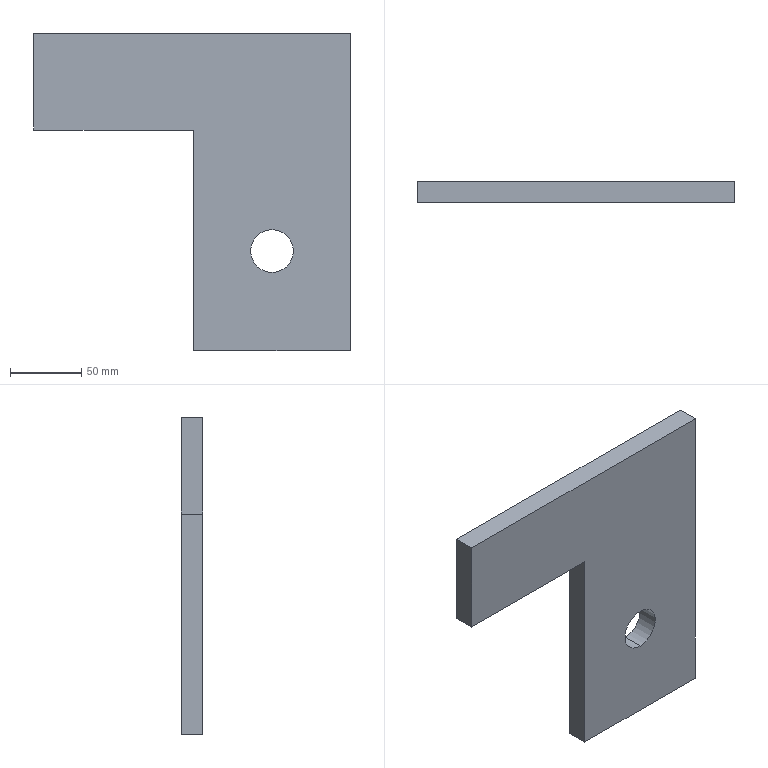Part | SolidWorks | features BaseBody 1 | 1 solid | 10 faces | box 222.333 x 15 x 223.043 mm | volume 471998 mm3 | plane 8 | cylinder 2 | commonest cylinder face diameters 30 x2
STEP:
#1=CARTESIAN_POINT('',(57.247,354.5,-81.));
#2=VERTEX_POINT('',#1);
#3=CARTESIAN_POINT('',(57.247,354.5,-51.));
#4=VERTEX_POINT('',#3);
#5=CARTESIAN_POINT('',(57.247,354.5,-66.));
#6=DIRECTION('',(0.,1.,0.));
#7=DIRECTION('',(0.,0.,1.));
#8=AXIS2_PLACEMENT_3D('',#5,#6,#7);
#9=CIRCLE('',#8,15.);
#10=EDGE_CURVE('',#2,#4,#9,.T.);
#11=ORIENTED_EDGE('',*,*,#10,.F.);
#12=CARTESIAN_POINT('',(57.247,369.5,-81.));
#13=VERTEX_POINT('',#12);
#14=CARTESIAN_POINT('',(57.247,389.5,-81.));
#15=DIRECTION('',(0.,1.,0.));
#16=VECTOR('',#15,1000.);
#17=LINE('',#14,#16);
#18=EDGE_CURVE('',#2,#13,#17,.T.);
#19=ORIENTED_EDGE('',*,*,#18,.T.);
#20=CARTESIAN_POINT('',(57.247,369.5,-51.));
#21=VERTEX_POINT('',#20);
#22=CARTESIAN_POINT('',(57.247,369.5,-66.));
#23=DIRECTION('',(0.,-1.,0.));
#24=DIRECTION('',(0.,0.,1.));
#25=AXIS2_PLACEMENT_3D('',#22,#23,#24);
#26=CIRCLE('',#25,15.);
#27=EDGE_CURVE('',#21,#13,#26,.T.);
#28=ORIENTED_EDGE('',*,*,#27,.F.);
#29=CARTESIAN_POINT('',(57.247,389.5,-51.));
#30=DIRECTION('',(0.,1.,0.));
#31=VECTOR('',#30,1000.);
#32=LINE('',#29,#31);
#33=EDGE_CURVE('',#4,#21,#32,.T.);
#34=ORIENTED_EDGE('',*,*,#33,.F.);
#35=EDGE_LOOP('',(#11,#19,#28,#34));
#36=FACE_OUTER_BOUND('',#35,.T.);
#37=CARTESIAN_POINT('',(57.247,389.5,-66.));
#38=DIRECTION('',(0.,1.,0.));
#39=DIRECTION('',(0.,0.,1.));
#40=AXIS2_PLACEMENT_3D('',#37,#38,#39);
#41=CYLINDRICAL_SURFACE('',#40,15.);
#42=ADVANCED_FACE('',(#36),#41,.F.);
#43=ORIENTED_EDGE('',*,*,#27,.T.);
#44=CARTESIAN_POINT('',(57.247,369.5,-66.));
#45=DIRECTION('',(0.,-1.,0.));
#46=DIRECTION('',(0.,0.,1.));
#47=AXIS2_PLACEMENT_3D('',#44,#45,#46);
#48=CIRCLE('',#47,15.);
#49=EDGE_CURVE('',#13,#21,#48,.T.);
#50=ORIENTED_EDGE('',*,*,#49,.T.);
#51=EDGE_LOOP('',(#43,#50));
#52=FACE_BOUND('',#51,.T.);
#53=CARTESIAN_POINT('',(112.247,369.5,-136.043));
#54=VERTEX_POINT('',#53);
#55=CARTESIAN_POINT('',(2.247,369.5,-136.043));
#56=VERTEX_POINT('',#55);
#57=CARTESIAN_POINT('',(57.247,369.5,-136.043));
#58=DIRECTION('',(-1.,0.,0.));
#59=VECTOR('',#58,1000.);
#60=LINE('',#57,#59);
#61=EDGE_CURVE('',#54,#56,#60,.T.);
#62=ORIENTED_EDGE('',*,*,#61,.T.);
#63=CARTESIAN_POINT('',(2.247,369.5,19.));
#64=VERTEX_POINT('',#63);
#65=CARTESIAN_POINT('',(2.247,369.5,-16.043));
#66=DIRECTION('',(0.,0.,1.));
#67=VECTOR('',#66,1000.);
#68=LINE('',#65,#67);
#69=EDGE_CURVE('',#56,#64,#68,.T.);
#70=ORIENTED_EDGE('',*,*,#69,.T.);
#71=CARTESIAN_POINT('',(-110.086,369.5,19.));
#72=VERTEX_POINT('',#71);
#73=CARTESIAN_POINT('',(57.247,369.5,19.));
#74=DIRECTION('',(-1.,0.,0.));
#75=VECTOR('',#74,1000.);
#76=LINE('',#73,#75);
#77=EDGE_CURVE('',#64,#72,#76,.T.);
#78=ORIENTED_EDGE('',*,*,#77,.T.);
#79=CARTESIAN_POINT('',(-110.086,369.5,87.));
#80=VERTEX_POINT('',#79);
#81=CARTESIAN_POINT('',(-110.086,369.5,-16.043));
#82=DIRECTION('',(0.,0.,1.));
#83=VECTOR('',#82,1000.);
#84=LINE('',#81,#83);
#85=EDGE_CURVE('',#72,#80,#84,.T.);
#86=ORIENTED_EDGE('',*,*,#85,.T.);
#87=CARTESIAN_POINT('',(112.247,369.5,87.));
#88=VERTEX_POINT('',#87);
#89=CARTESIAN_POINT('',(57.247,369.5,87.));
#90=DIRECTION('',(1.,0.,0.));
#91=VECTOR('',#90,1000.);
#92=LINE('',#89,#91);
#93=EDGE_CURVE('',#80,#88,#92,.T.);
#94=ORIENTED_EDGE('',*,*,#93,.T.);
#95=CARTESIAN_POINT('',(112.247,369.5,-16.043));
#96=DIRECTION('',(0.,0.,-1.));
#97=VECTOR('',#96,1000.);
#98=LINE('',#95,#97);
#99=EDGE_CURVE('',#88,#54,#98,.T.);
#100=ORIENTED_EDGE('',*,*,#99,.T.);
#101=EDGE_LOOP('',(#62,#70,#78,#86,#94,#100));
#102=FACE_OUTER_BOUND('',#101,.T.);
#103=CARTESIAN_POINT('',(57.247,369.5,-16.043));
#104=DIRECTION('',(0.,1.,0.));
#105=DIRECTION('',(0.,0.,1.));
#106=AXIS2_PLACEMENT_3D('',#103,#104,#105);
#107=PLANE('',#106);
#108=ADVANCED_FACE('',(#52,#102),#107,.T.);
#109=ORIENTED_EDGE('',*,*,#18,.F.);
#110=CARTESIAN_POINT('',(57.247,354.5,-66.));
#111=DIRECTION('',(0.,1.,0.));
#112=DIRECTION('',(0.,0.,1.));
#113=AXIS2_PLACEMENT_3D('',#110,#111,#112);
#114=CIRCLE('',#113,15.);
#115=EDGE_CURVE('',#4,#2,#114,.T.);
#116=ORIENTED_EDGE('',*,*,#115,.F.);
#117=ORIENTED_EDGE('',*,*,#33,.T.);
#118=ORIENTED_EDGE('',*,*,#49,.F.);
#119=EDGE_LOOP('',(#109,#116,#117,#118));
#120=FACE_OUTER_BOUND('',#119,.T.);
#121=CARTESIAN_POINT('',(57.247,389.5,-66.));
#122=DIRECTION('',(0.,1.,0.));
#123=DIRECTION('',(0.,0.,1.));
#124=AXIS2_PLACEMENT_3D('',#121,#122,#123);
#125=CYLINDRICAL_SURFACE('',#124,15.);
#126=ADVANCED_FACE('',(#120),#125,.F.);
#127=CARTESIAN_POINT('',(2.247,354.5,-136.043));
#128=VERTEX_POINT('',#127);
#129=CARTESIAN_POINT('',(2.247,354.5,19.));
#130=VERTEX_POINT('',#129);
#131=CARTESIAN_POINT('',(2.247,354.5,-16.043));
#132=DIRECTION('',(0.,0.,1.));
#133=VECTOR('',#132,1000.);
#134=LINE('',#131,#133);
#135=EDGE_CURVE('',#128,#130,#134,.T.);
#136=ORIENTED_EDGE('',*,*,#135,.T.);
#137=CARTESIAN_POINT('',(2.247,357.,19.));
#138=DIRECTION('',(0.,1.,0.));
#139=VECTOR('',#138,1000.);
#140=LINE('',#137,#139);
#141=EDGE_CURVE('',#130,#64,#140,.T.);
#142=ORIENTED_EDGE('',*,*,#141,.T.);
#143=ORIENTED_EDGE('',*,*,#69,.F.);
#144=CARTESIAN_POINT('',(2.247,357.,-136.043));
#145=DIRECTION('',(0.,-1.,0.));
#146=VECTOR('',#145,1000.);
#147=LINE('',#144,#146);
#148=EDGE_CURVE('',#56,#128,#147,.T.);
#149=ORIENTED_EDGE('',*,*,#148,.T.);
#150=EDGE_LOOP('',(#136,#142,#143,#149));
#151=FACE_OUTER_BOUND('',#150,.T.);
#152=CARTESIAN_POINT('',(2.247,357.,-16.043));
#153=DIRECTION('',(-1.,0.,0.));
#154=DIRECTION('',(0.,0.,1.));
#155=AXIS2_PLACEMENT_3D('',#152,#153,#154);
#156=PLANE('',#155);
#157=ADVANCED_FACE('',(#151),#156,.T.);
#158=ORIENTED_EDGE('',*,*,#61,.F.);
#159=CARTESIAN_POINT('',(112.247,354.5,-136.043));
#160=VERTEX_POINT('',#159);
#161=CARTESIAN_POINT('',(112.247,357.,-136.043));
#162=DIRECTION('',(0.,1.,0.));
#163=VECTOR('',#162,1000.);
#164=LINE('',#161,#163);
#165=EDGE_CURVE('',#160,#54,#164,.T.);
#166=ORIENTED_EDGE('',*,*,#165,.F.);
#167=CARTESIAN_POINT('',(57.247,354.5,-136.043));
#168=DIRECTION('',(1.,0.,0.));
#169=VECTOR('',#168,1000.);
#170=LINE('',#167,#169);
#171=EDGE_CURVE('',#128,#160,#170,.T.);
#172=ORIENTED_EDGE('',*,*,#171,.F.);
#173=ORIENTED_EDGE('',*,*,#148,.F.);
#174=EDGE_LOOP('',(#158,#166,#172,#173));
#175=FACE_OUTER_BOUND('',#174,.T.);
#176=CARTESIAN_POINT('',(57.247,357.,-136.043));
#177=DIRECTION('',(0.,0.,1.));
#178=DIRECTION('',(1.,0.,0.));
#179=AXIS2_PLACEMENT_3D('',#176,#177,#178);
#180=PLANE('',#179);
#181=ADVANCED_FACE('',(#175),#180,.F.);
#182=ORIENTED_EDGE('',*,*,#165,.T.);
#183=ORIENTED_EDGE('',*,*,#99,.F.);
#184=CARTESIAN_POINT('',(112.247,354.5,87.));
#185=VERTEX_POINT('',#184);
#186=CARTESIAN_POINT('',(112.247,357.,87.));
#187=DIRECTION('',(0.,-1.,0.));
#188=VECTOR('',#187,1000.);
#189=LINE('',#186,#188);
#190=EDGE_CURVE('',#88,#185,#189,.T.);
#191=ORIENTED_EDGE('',*,*,#190,.T.);
#192=CARTESIAN_POINT('',(112.247,354.5,-16.043));
#193=DIRECTION('',(0.,0.,-1.));
#194=VECTOR('',#193,1000.);
#195=LINE('',#192,#194);
#196=EDGE_CURVE('',#185,#160,#195,.T.);
#197=ORIENTED_EDGE('',*,*,#196,.T.);
#198=EDGE_LOOP('',(#182,#183,#191,#197));
#199=FACE_OUTER_BOUND('',#198,.T.);
#200=CARTESIAN_POINT('',(112.247,357.,-16.043));
#201=DIRECTION('',(1.,0.,0.));
#202=DIRECTION('',(0.,0.,-1.));
#203=AXIS2_PLACEMENT_3D('',#200,#201,#202);
#204=PLANE('',#203);
#205=ADVANCED_FACE('',(#199),#204,.T.);
#206=CARTESIAN_POINT('',(-110.086,354.5,87.));
#207=VERTEX_POINT('',#206);
#208=CARTESIAN_POINT('',(-110.086,381.4,87.));
#209=DIRECTION('',(0.,1.,0.));
#210=VECTOR('',#209,1000.);
#211=LINE('',#208,#210);
#212=EDGE_CURVE('',#207,#80,#211,.T.);
#213=ORIENTED_EDGE('',*,*,#212,.F.);
#214=CARTESIAN_POINT('',(-116.886,354.5,87.));
#215=DIRECTION('',(-1.,0.,0.));
#216=VECTOR('',#215,1000.);
#217=LINE('',#214,#216);
#218=EDGE_CURVE('',#185,#207,#217,.T.);
#219=ORIENTED_EDGE('',*,*,#218,.F.);
#220=ORIENTED_EDGE('',*,*,#190,.F.);
#221=ORIENTED_EDGE('',*,*,#93,.F.);
#222=EDGE_LOOP('',(#213,#219,#220,#221));
#223=FACE_OUTER_BOUND('',#222,.T.);
#224=CARTESIAN_POINT('',(-116.886,381.4,87.));
#225=DIRECTION('',(0.,0.,-1.));
#226=DIRECTION('',(-1.,0.,0.));
#227=AXIS2_PLACEMENT_3D('',#224,#225,#226);
#228=PLANE('',#227);
#229=ADVANCED_FACE('',(#223),#228,.F.);
#230=CARTESIAN_POINT('',(-110.086,354.5,19.));
#231=VERTEX_POINT('',#230);
#232=CARTESIAN_POINT('',(-110.086,354.5,78.6));
#233=DIRECTION('',(0.,0.,-1.));
#234=VECTOR('',#233,1000.);
#235=LINE('',#232,#234);
#236=EDGE_CURVE('',#207,#231,#235,.T.);
#237=ORIENTED_EDGE('',*,*,#236,.F.);
#238=ORIENTED_EDGE('',*,*,#212,.T.);
#239=ORIENTED_EDGE('',*,*,#85,.F.);
#240=CARTESIAN_POINT('',(-110.086,408.2,19.));
#241=DIRECTION('',(0.,1.,0.));
#242=VECTOR('',#241,1000.);
#243=LINE('',#240,#242);
#244=EDGE_CURVE('',#231,#72,#243,.T.);
#245=ORIENTED_EDGE('',*,*,#244,.F.);
#246=EDGE_LOOP('',(#237,#238,#239,#245));
#247=FACE_OUTER_BOUND('',#246,.T.);
#248=CARTESIAN_POINT('',(-110.086,408.2,78.6));
#249=DIRECTION('',(1.,0.,0.));
#250=DIRECTION('',(0.,0.,-1.));
#251=AXIS2_PLACEMENT_3D('',#248,#249,#250);
#252=PLANE('',#251);
#253=ADVANCED_FACE('',(#247),#252,.F.);
#254=ORIENTED_EDGE('',*,*,#244,.T.);
#255=ORIENTED_EDGE('',*,*,#77,.F.);
#256=ORIENTED_EDGE('',*,*,#141,.F.);
#257=CARTESIAN_POINT('',(-76.886,354.5,19.));
#258=DIRECTION('',(-1.,0.,0.));
#259=VECTOR('',#258,1000.);
#260=LINE('',#257,#259);
#261=EDGE_CURVE('',#130,#231,#260,.T.);
#262=ORIENTED_EDGE('',*,*,#261,.T.);
#263=EDGE_LOOP('',(#254,#255,#256,#262));
#264=FACE_OUTER_BOUND('',#263,.T.);
#265=CARTESIAN_POINT('',(-76.886,407.,19.));
#266=DIRECTION('',(0.,0.,-1.));
#267=DIRECTION('',(-1.,0.,0.));
#268=AXIS2_PLACEMENT_3D('',#265,#266,#267);
#269=PLANE('',#268);
#270=ADVANCED_FACE('',(#264),#269,.T.);
#271=ORIENTED_EDGE('',*,*,#115,.T.);
#272=ORIENTED_EDGE('',*,*,#10,.T.);
#273=EDGE_LOOP('',(#271,#272));
#274=FACE_BOUND('',#273,.T.);
#275=ORIENTED_EDGE('',*,*,#171,.T.);
#276=ORIENTED_EDGE('',*,*,#196,.F.);
#277=ORIENTED_EDGE('',*,*,#218,.T.);
#278=ORIENTED_EDGE('',*,*,#236,.T.);
#279=ORIENTED_EDGE('',*,*,#261,.F.);
#280=ORIENTED_EDGE('',*,*,#135,.F.);
#281=EDGE_LOOP('',(#275,#276,#277,#278,#279,#280));
#282=FACE_OUTER_BOUND('',#281,.T.);
#283=CARTESIAN_POINT('',(31.631,354.5,-284.615));
#284=DIRECTION('',(0.,-1.,0.));
#285=DIRECTION('',(0.,0.,-1.));
#286=AXIS2_PLACEMENT_3D('',#283,#284,#285);
#287=PLANE('',#286);
#288=ADVANCED_FACE('',(#274,#282),#287,.T.);
#289=CLOSED_SHELL('',(#42,#108,#126,#157,#181,#205,#229,#253,#270,#288));
#290=MANIFOLD_SOLID_BREP('',#289);
#291=CARTESIAN_POINT('',(0.,0.,0.));
#292=DIRECTION('',(0.,0.,1.));
#293=DIRECTION('',(1.,0.,0.));
#294=AXIS2_PLACEMENT_3D('',#291,#292,#293);
#295=(LENGTH_UNIT()NAMED_UNIT(*)SI_UNIT(.MILLI.,.METRE.));
#296=UNCERTAINTY_MEASURE_WITH_UNIT(LENGTH_MEASURE(0.00001),#295,'','');
#297=(NAMED_UNIT(*)PLANE_ANGLE_UNIT()SI_UNIT($,.RADIAN.));
#298=(NAMED_UNIT(*)SI_UNIT($,.STERADIAN.)SOLID_ANGLE_UNIT());
#299=(GEOMETRIC_REPRESENTATION_CONTEXT(3)GLOBAL_UNCERTAINTY_ASSIGNED_CONTEXT((#296))GLOBAL_UNIT_ASSIGNED_CONTEXT((#295,#297,#298))REPRESENTATION_CONTEXT('',''));
#300=ADVANCED_BREP_SHAPE_REPRESENTATION('',(#290,#294),#299);